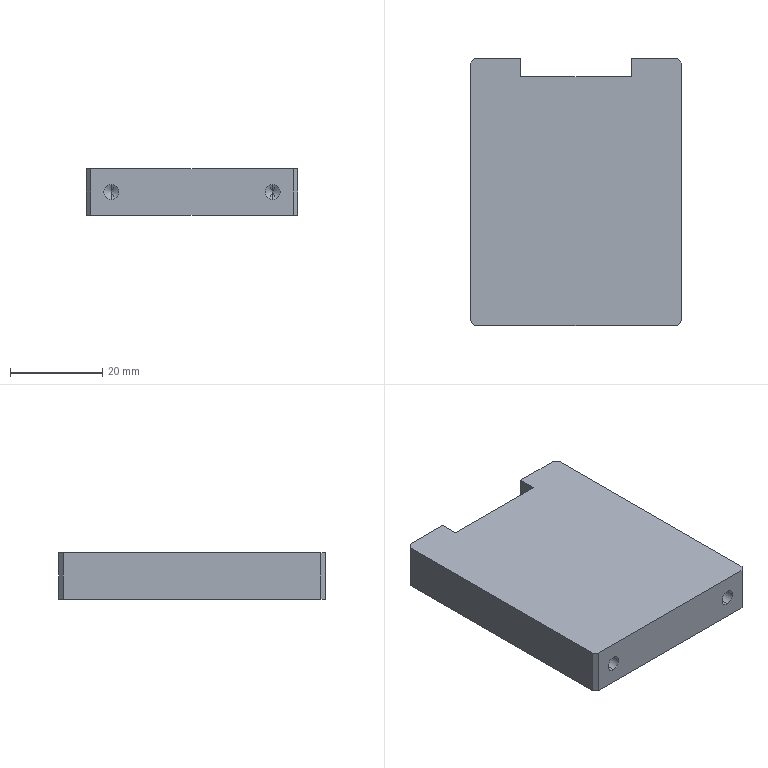Part | NX | features BREP 1 | 1 solid | 22 faces | box 46 x 58 x 10 mm | volume 25498 mm3 | plane 14 | cylinder 4 | cone 4 | commonest cylinder face diameters 3.3 x4
STEP:
#1=CARTESIAN_POINT('',(-17.5,-17.5,1.65));
#2=VERTEX_POINT('',#1);
#3=CARTESIAN_POINT('',(-17.5,-17.5,-1.65));
#4=VERTEX_POINT('',#3);
#5=CARTESIAN_POINT('',(-17.5,-17.5,0.));
#6=DIRECTION('',(0.,-1.,0.));
#7=DIRECTION('',(0.,0.,-1.));
#8=AXIS2_PLACEMENT_3D('',#5,#6,#7);
#9=CIRCLE('',#8,1.65);
#10=EDGE_CURVE('',#2,#4,#9,.T.);
#11=ORIENTED_EDGE('',*,*,#10,.F.);
#12=CARTESIAN_POINT('',(-17.5,-29.,1.65));
#13=VERTEX_POINT('',#12);
#14=CARTESIAN_POINT('',(-17.5,-29.,1.65));
#15=DIRECTION('',(0.,-1.,0.));
#16=VECTOR('',#15,1000.);
#17=LINE('',#14,#16);
#18=EDGE_CURVE('',#2,#13,#17,.T.);
#19=ORIENTED_EDGE('',*,*,#18,.T.);
#20=CARTESIAN_POINT('',(-17.5,-29.,-1.65));
#21=VERTEX_POINT('',#20);
#22=CARTESIAN_POINT('',(-17.5,-29.,0.));
#23=DIRECTION('',(0.,-1.,0.));
#24=DIRECTION('',(0.,0.,-1.));
#25=AXIS2_PLACEMENT_3D('',#22,#23,#24);
#26=CIRCLE('',#25,1.65);
#27=EDGE_CURVE('',#13,#21,#26,.T.);
#28=ORIENTED_EDGE('',*,*,#27,.T.);
#29=CARTESIAN_POINT('',(-17.5,-29.,-1.65));
#30=DIRECTION('',(0.,-1.,0.));
#31=VECTOR('',#30,1000.);
#32=LINE('',#29,#31);
#33=EDGE_CURVE('',#4,#21,#32,.T.);
#34=ORIENTED_EDGE('',*,*,#33,.F.);
#35=EDGE_LOOP('',(#11,#19,#28,#34));
#36=FACE_BOUND('',#35,.T.);
#37=CARTESIAN_POINT('',(-17.5,-29.,0.));
#38=DIRECTION('',(0.,-1.,0.));
#39=DIRECTION('',(0.,0.,-1.));
#40=AXIS2_PLACEMENT_3D('',#37,#38,#39);
#41=CYLINDRICAL_SURFACE('',#40,1.65);
#42=ADVANCED_FACE('',(#36),#41,.F.);
#43=CARTESIAN_POINT('',(-17.5,-16.509,0.));
#44=VERTEX_POINT('',#43);
#45=CARTESIAN_POINT('',(-17.5,-17.5,-1.65));
#46=DIRECTION('',(0.,-0.515,-0.8572));
#47=VECTOR('',#46,1000.);
#48=LINE('',#45,#47);
#49=EDGE_CURVE('',#44,#4,#48,.T.);
#50=ORIENTED_EDGE('',*,*,#49,.F.);
#51=CARTESIAN_POINT('',(-17.5,-17.5,1.65));
#52=DIRECTION('',(0.,-0.515,0.8572));
#53=VECTOR('',#52,1000.);
#54=LINE('',#51,#53);
#55=EDGE_CURVE('',#44,#2,#54,.T.);
#56=ORIENTED_EDGE('',*,*,#55,.T.);
#57=ORIENTED_EDGE('',*,*,#10,.T.);
#58=EDGE_LOOP('',(#50,#56,#57));
#59=FACE_BOUND('',#58,.T.);
#60=CARTESIAN_POINT('',(-17.5,-17.5,0.));
#61=DIRECTION('',(0.,-1.,0.));
#62=DIRECTION('',(0.,0.,-1.));
#63=AXIS2_PLACEMENT_3D('',#60,#61,#62);
#64=CONICAL_SURFACE('',#63,1.65,1.03);
#65=ADVANCED_FACE('',(#59),#64,.F.);
#66=CARTESIAN_POINT('',(17.5,-17.5,1.65));
#67=VERTEX_POINT('',#66);
#68=CARTESIAN_POINT('',(17.5,-17.5,-1.65));
#69=VERTEX_POINT('',#68);
#70=CARTESIAN_POINT('',(17.5,-17.5,0.));
#71=DIRECTION('',(0.,-1.,0.));
#72=DIRECTION('',(0.,0.,-1.));
#73=AXIS2_PLACEMENT_3D('',#70,#71,#72);
#74=CIRCLE('',#73,1.65);
#75=EDGE_CURVE('',#67,#69,#74,.T.);
#76=ORIENTED_EDGE('',*,*,#75,.F.);
#77=CARTESIAN_POINT('',(17.5,-29.,1.65));
#78=VERTEX_POINT('',#77);
#79=CARTESIAN_POINT('',(17.5,-29.,1.65));
#80=DIRECTION('',(0.,-1.,0.));
#81=VECTOR('',#80,1000.);
#82=LINE('',#79,#81);
#83=EDGE_CURVE('',#67,#78,#82,.T.);
#84=ORIENTED_EDGE('',*,*,#83,.T.);
#85=CARTESIAN_POINT('',(17.5,-29.,-1.65));
#86=VERTEX_POINT('',#85);
#87=CARTESIAN_POINT('',(17.5,-29.,0.));
#88=DIRECTION('',(0.,-1.,0.));
#89=DIRECTION('',(0.,0.,-1.));
#90=AXIS2_PLACEMENT_3D('',#87,#88,#89);
#91=CIRCLE('',#90,1.65);
#92=EDGE_CURVE('',#78,#86,#91,.T.);
#93=ORIENTED_EDGE('',*,*,#92,.T.);
#94=CARTESIAN_POINT('',(17.5,-29.,-1.65));
#95=DIRECTION('',(0.,-1.,0.));
#96=VECTOR('',#95,1000.);
#97=LINE('',#94,#96);
#98=EDGE_CURVE('',#69,#86,#97,.T.);
#99=ORIENTED_EDGE('',*,*,#98,.F.);
#100=EDGE_LOOP('',(#76,#84,#93,#99));
#101=FACE_BOUND('',#100,.T.);
#102=CARTESIAN_POINT('',(17.5,-29.,0.));
#103=DIRECTION('',(0.,-1.,0.));
#104=DIRECTION('',(0.,0.,-1.));
#105=AXIS2_PLACEMENT_3D('',#102,#103,#104);
#106=CYLINDRICAL_SURFACE('',#105,1.65);
#107=ADVANCED_FACE('',(#101),#106,.F.);
#108=CARTESIAN_POINT('',(17.5,-16.509,0.));
#109=VERTEX_POINT('',#108);
#110=CARTESIAN_POINT('',(17.5,-17.5,-1.65));
#111=DIRECTION('',(0.,-0.515,-0.8572));
#112=VECTOR('',#111,1000.);
#113=LINE('',#110,#112);
#114=EDGE_CURVE('',#109,#69,#113,.T.);
#115=ORIENTED_EDGE('',*,*,#114,.F.);
#116=CARTESIAN_POINT('',(17.5,-17.5,1.65));
#117=DIRECTION('',(0.,-0.515,0.8572));
#118=VECTOR('',#117,1000.);
#119=LINE('',#116,#118);
#120=EDGE_CURVE('',#109,#67,#119,.T.);
#121=ORIENTED_EDGE('',*,*,#120,.T.);
#122=ORIENTED_EDGE('',*,*,#75,.T.);
#123=EDGE_LOOP('',(#115,#121,#122));
#124=FACE_BOUND('',#123,.T.);
#125=CARTESIAN_POINT('',(17.5,-17.5,0.));
#126=DIRECTION('',(0.,-1.,0.));
#127=DIRECTION('',(0.,0.,-1.));
#128=AXIS2_PLACEMENT_3D('',#125,#126,#127);
#129=CONICAL_SURFACE('',#128,1.65,1.03);
#130=ADVANCED_FACE('',(#124),#129,.F.);
#131=CARTESIAN_POINT('',(22.,29.,5.));
#132=VERTEX_POINT('',#131);
#133=CARTESIAN_POINT('',(12.,29.,5.));
#134=VERTEX_POINT('',#133);
#135=CARTESIAN_POINT('',(23.,29.,5.));
#136=DIRECTION('',(-1.,0.,0.));
#137=VECTOR('',#136,1000.);
#138=LINE('',#135,#137);
#139=EDGE_CURVE('',#132,#134,#138,.T.);
#140=ORIENTED_EDGE('',*,*,#139,.F.);
#141=CARTESIAN_POINT('',(22.,29.,-5.));
#142=VERTEX_POINT('',#141);
#143=CARTESIAN_POINT('',(22.,29.,5.));
#144=DIRECTION('',(0.,0.,-1.));
#145=VECTOR('',#144,1000.);
#146=LINE('',#143,#145);
#147=EDGE_CURVE('',#132,#142,#146,.T.);
#148=ORIENTED_EDGE('',*,*,#147,.T.);
#149=CARTESIAN_POINT('',(12.,29.,-5.));
#150=VERTEX_POINT('',#149);
#151=CARTESIAN_POINT('',(23.,29.,-5.));
#152=DIRECTION('',(-1.,0.,0.));
#153=VECTOR('',#152,1000.);
#154=LINE('',#151,#153);
#155=EDGE_CURVE('',#142,#150,#154,.T.);
#156=ORIENTED_EDGE('',*,*,#155,.T.);
#157=CARTESIAN_POINT('',(12.,29.,-5.));
#158=DIRECTION('',(0.,0.,-1.));
#159=VECTOR('',#158,1000.);
#160=LINE('',#157,#159);
#161=EDGE_CURVE('',#134,#150,#160,.T.);
#162=ORIENTED_EDGE('',*,*,#161,.F.);
#163=EDGE_LOOP('',(#140,#148,#156,#162));
#164=FACE_BOUND('',#163,.T.);
#165=CARTESIAN_POINT('',(23.,29.,5.));
#166=DIRECTION('',(0.,-1.,0.));
#167=DIRECTION('',(0.,0.,-1.));
#168=AXIS2_PLACEMENT_3D('',#165,#166,#167);
#169=PLANE('',#168);
#170=ADVANCED_FACE('',(#164),#169,.F.);
#171=CARTESIAN_POINT('',(-23.,28.,-5.));
#172=VERTEX_POINT('',#171);
#173=CARTESIAN_POINT('',(-23.,-28.,-5.));
#174=VERTEX_POINT('',#173);
#175=CARTESIAN_POINT('',(-23.,-29.,-5.));
#176=DIRECTION('',(0.,-1.,0.));
#177=VECTOR('',#176,1000.);
#178=LINE('',#175,#177);
#179=EDGE_CURVE('',#172,#174,#178,.T.);
#180=ORIENTED_EDGE('',*,*,#179,.T.);
#181=CARTESIAN_POINT('',(-23.,-28.,5.));
#182=VERTEX_POINT('',#181);
#183=CARTESIAN_POINT('',(-23.,-28.,5.));
#184=DIRECTION('',(0.,0.,1.));
#185=VECTOR('',#184,1000.);
#186=LINE('',#183,#185);
#187=EDGE_CURVE('',#174,#182,#186,.T.);
#188=ORIENTED_EDGE('',*,*,#187,.T.);
#189=CARTESIAN_POINT('',(-23.,28.,5.));
#190=VERTEX_POINT('',#189);
#191=CARTESIAN_POINT('',(-23.,-29.,5.));
#192=DIRECTION('',(0.,-1.,0.));
#193=VECTOR('',#192,1000.);
#194=LINE('',#191,#193);
#195=EDGE_CURVE('',#190,#182,#194,.T.);
#196=ORIENTED_EDGE('',*,*,#195,.F.);
#197=CARTESIAN_POINT('',(-23.,28.,5.));
#198=DIRECTION('',(0.,0.,-1.));
#199=VECTOR('',#198,1000.);
#200=LINE('',#197,#199);
#201=EDGE_CURVE('',#190,#172,#200,.T.);
#202=ORIENTED_EDGE('',*,*,#201,.T.);
#203=EDGE_LOOP('',(#180,#188,#196,#202));
#204=FACE_BOUND('',#203,.T.);
#205=CARTESIAN_POINT('',(-23.,-29.,5.));
#206=DIRECTION('',(1.,0.,0.));
#207=DIRECTION('',(0.,1.,0.));
#208=AXIS2_PLACEMENT_3D('',#205,#206,#207);
#209=PLANE('',#208);
#210=ADVANCED_FACE('',(#204),#209,.F.);
#211=CARTESIAN_POINT('',(-22.,-29.,5.));
#212=VERTEX_POINT('',#211);
#213=CARTESIAN_POINT('',(22.,-29.,5.));
#214=VERTEX_POINT('',#213);
#215=CARTESIAN_POINT('',(23.,-29.,5.));
#216=DIRECTION('',(1.,0.,0.));
#217=VECTOR('',#216,1000.);
#218=LINE('',#215,#217);
#219=EDGE_CURVE('',#212,#214,#218,.T.);
#220=ORIENTED_EDGE('',*,*,#219,.F.);
#221=CARTESIAN_POINT('',(-22.,-29.,-5.));
#222=VERTEX_POINT('',#221);
#223=CARTESIAN_POINT('',(-22.,-29.,5.));
#224=DIRECTION('',(0.,0.,-1.));
#225=VECTOR('',#224,1000.);
#226=LINE('',#223,#225);
#227=EDGE_CURVE('',#212,#222,#226,.T.);
#228=ORIENTED_EDGE('',*,*,#227,.T.);
#229=CARTESIAN_POINT('',(22.,-29.,-5.));
#230=VERTEX_POINT('',#229);
#231=CARTESIAN_POINT('',(23.,-29.,-5.));
#232=DIRECTION('',(1.,0.,0.));
#233=VECTOR('',#232,1000.);
#234=LINE('',#231,#233);
#235=EDGE_CURVE('',#222,#230,#234,.T.);
#236=ORIENTED_EDGE('',*,*,#235,.T.);
#237=CARTESIAN_POINT('',(22.,-29.,5.));
#238=DIRECTION('',(0.,0.,1.));
#239=VECTOR('',#238,1000.);
#240=LINE('',#237,#239);
#241=EDGE_CURVE('',#230,#214,#240,.T.);
#242=ORIENTED_EDGE('',*,*,#241,.T.);
#243=EDGE_LOOP('',(#220,#228,#236,#242));
#244=FACE_BOUND('',#243,.T.);
#245=CARTESIAN_POINT('',(-17.5,-29.,0.));
#246=DIRECTION('',(0.,-1.,0.));
#247=DIRECTION('',(0.,0.,-1.));
#248=AXIS2_PLACEMENT_3D('',#245,#246,#247);
#249=CIRCLE('',#248,1.65);
#250=EDGE_CURVE('',#21,#13,#249,.T.);
#251=ORIENTED_EDGE('',*,*,#250,.F.);
#252=ORIENTED_EDGE('',*,*,#27,.F.);
#253=EDGE_LOOP('',(#251,#252));
#254=FACE_BOUND('',#253,.T.);
#255=CARTESIAN_POINT('',(17.5,-29.,0.));
#256=DIRECTION('',(0.,-1.,0.));
#257=DIRECTION('',(0.,0.,-1.));
#258=AXIS2_PLACEMENT_3D('',#255,#256,#257);
#259=CIRCLE('',#258,1.65);
#260=EDGE_CURVE('',#86,#78,#259,.T.);
#261=ORIENTED_EDGE('',*,*,#260,.F.);
#262=ORIENTED_EDGE('',*,*,#92,.F.);
#263=EDGE_LOOP('',(#261,#262));
#264=FACE_BOUND('',#263,.T.);
#265=CARTESIAN_POINT('',(23.,-29.,5.));
#266=DIRECTION('',(0.,1.,0.));
#267=DIRECTION('',(1.,0.,0.));
#268=AXIS2_PLACEMENT_3D('',#265,#266,#267);
#269=PLANE('',#268);
#270=ADVANCED_FACE('',(#244,#254,#264),#269,.F.);
#271=CARTESIAN_POINT('',(23.,-28.,5.));
#272=VERTEX_POINT('',#271);
#273=CARTESIAN_POINT('',(23.,28.,5.));
#274=VERTEX_POINT('',#273);
#275=CARTESIAN_POINT('',(23.,-29.,5.));
#276=DIRECTION('',(0.,1.,0.));
#277=VECTOR('',#276,1000.);
#278=LINE('',#275,#277);
#279=EDGE_CURVE('',#272,#274,#278,.T.);
#280=ORIENTED_EDGE('',*,*,#279,.F.);
#281=CARTESIAN_POINT('',(23.,-28.,-5.));
#282=VERTEX_POINT('',#281);
#283=CARTESIAN_POINT('',(23.,-28.,5.));
#284=DIRECTION('',(0.,0.,-1.));
#285=VECTOR('',#284,1000.);
#286=LINE('',#283,#285);
#287=EDGE_CURVE('',#272,#282,#286,.T.);
#288=ORIENTED_EDGE('',*,*,#287,.T.);
#289=CARTESIAN_POINT('',(23.,28.,-5.));
#290=VERTEX_POINT('',#289);
#291=CARTESIAN_POINT('',(23.,-29.,-5.));
#292=DIRECTION('',(0.,1.,0.));
#293=VECTOR('',#292,1000.);
#294=LINE('',#291,#293);
#295=EDGE_CURVE('',#282,#290,#294,.T.);
#296=ORIENTED_EDGE('',*,*,#295,.T.);
#297=CARTESIAN_POINT('',(23.,28.,5.));
#298=DIRECTION('',(0.,0.,1.));
#299=VECTOR('',#298,1000.);
#300=LINE('',#297,#299);
#301=EDGE_CURVE('',#290,#274,#300,.T.);
#302=ORIENTED_EDGE('',*,*,#301,.T.);
#303=EDGE_LOOP('',(#280,#288,#296,#302));
#304=FACE_BOUND('',#303,.T.);
#305=CARTESIAN_POINT('',(23.,-29.,5.));
#306=DIRECTION('',(-1.,0.,0.));
#307=DIRECTION('',(0.,0.,1.));
#308=AXIS2_PLACEMENT_3D('',#305,#306,#307);
#309=PLANE('',#308);
#310=ADVANCED_FACE('',(#304),#309,.F.);
#311=CARTESIAN_POINT('',(-12.,29.,-5.));
#312=VERTEX_POINT('',#311);
#313=CARTESIAN_POINT('',(-22.,29.,-5.));
#314=VERTEX_POINT('',#313);
#315=CARTESIAN_POINT('',(23.,29.,-5.));
#316=DIRECTION('',(-1.,0.,0.));
#317=VECTOR('',#316,1000.);
#318=LINE('',#315,#317);
#319=EDGE_CURVE('',#312,#314,#318,.T.);
#320=ORIENTED_EDGE('',*,*,#319,.T.);
#321=CARTESIAN_POINT('',(-22.,29.,5.));
#322=VERTEX_POINT('',#321);
#323=CARTESIAN_POINT('',(-22.,29.,5.));
#324=DIRECTION('',(0.,0.,1.));
#325=VECTOR('',#324,1000.);
#326=LINE('',#323,#325);
#327=EDGE_CURVE('',#314,#322,#326,.T.);
#328=ORIENTED_EDGE('',*,*,#327,.T.);
#329=CARTESIAN_POINT('',(-12.,29.,5.));
#330=VERTEX_POINT('',#329);
#331=CARTESIAN_POINT('',(23.,29.,5.));
#332=DIRECTION('',(-1.,0.,0.));
#333=VECTOR('',#332,1000.);
#334=LINE('',#331,#333);
#335=EDGE_CURVE('',#330,#322,#334,.T.);
#336=ORIENTED_EDGE('',*,*,#335,.F.);
#337=CARTESIAN_POINT('',(-12.,29.,-5.));
#338=DIRECTION('',(0.,0.,1.));
#339=VECTOR('',#338,1000.);
#340=LINE('',#337,#339);
#341=EDGE_CURVE('',#312,#330,#340,.T.);
#342=ORIENTED_EDGE('',*,*,#341,.F.);
#343=EDGE_LOOP('',(#320,#328,#336,#342));
#344=FACE_BOUND('',#343,.T.);
#345=CARTESIAN_POINT('',(23.,29.,5.));
#346=DIRECTION('',(0.,-1.,0.));
#347=DIRECTION('',(0.,0.,-1.));
#348=AXIS2_PLACEMENT_3D('',#345,#346,#347);
#349=PLANE('',#348);
#350=ADVANCED_FACE('',(#344),#349,.F.);
#351=ORIENTED_EDGE('',*,*,#195,.T.);
#352=CARTESIAN_POINT('',(-25.5,-25.5,5.));
#353=DIRECTION('',(0.7071,-0.7071,0.));
#354=VECTOR('',#353,1000.);
#355=LINE('',#352,#354);
#356=EDGE_CURVE('',#182,#212,#355,.T.);
#357=ORIENTED_EDGE('',*,*,#356,.T.);
#358=ORIENTED_EDGE('',*,*,#219,.T.);
#359=CARTESIAN_POINT('',(25.5,-25.5,5.));
#360=DIRECTION('',(0.7071,0.7071,0.));
#361=VECTOR('',#360,1000.);
#362=LINE('',#359,#361);
#363=EDGE_CURVE('',#214,#272,#362,.T.);
#364=ORIENTED_EDGE('',*,*,#363,.T.);
#365=ORIENTED_EDGE('',*,*,#279,.T.);
#366=CARTESIAN_POINT('',(25.5,25.5,5.));
#367=DIRECTION('',(-0.7071,0.7071,0.));
#368=VECTOR('',#367,1000.);
#369=LINE('',#366,#368);
#370=EDGE_CURVE('',#274,#132,#369,.T.);
#371=ORIENTED_EDGE('',*,*,#370,.T.);
#372=ORIENTED_EDGE('',*,*,#139,.T.);
#373=CARTESIAN_POINT('',(12.,25.,5.));
#374=VERTEX_POINT('',#373);
#375=CARTESIAN_POINT('',(12.,25.,5.));
#376=DIRECTION('',(0.,1.,0.));
#377=VECTOR('',#376,1000.);
#378=LINE('',#375,#377);
#379=EDGE_CURVE('',#374,#134,#378,.T.);
#380=ORIENTED_EDGE('',*,*,#379,.F.);
#381=CARTESIAN_POINT('',(-12.,25.,5.));
#382=VERTEX_POINT('',#381);
#383=CARTESIAN_POINT('',(-12.,25.,5.));
#384=DIRECTION('',(1.,0.,0.));
#385=VECTOR('',#384,1000.);
#386=LINE('',#383,#385);
#387=EDGE_CURVE('',#382,#374,#386,.T.);
#388=ORIENTED_EDGE('',*,*,#387,.F.);
#389=CARTESIAN_POINT('',(-12.,25.,5.));
#390=DIRECTION('',(0.,1.,0.));
#391=VECTOR('',#390,1000.);
#392=LINE('',#389,#391);
#393=EDGE_CURVE('',#382,#330,#392,.T.);
#394=ORIENTED_EDGE('',*,*,#393,.T.);
#395=ORIENTED_EDGE('',*,*,#335,.T.);
#396=CARTESIAN_POINT('',(-25.5,25.5,5.));
#397=DIRECTION('',(-0.7071,-0.7071,0.));
#398=VECTOR('',#397,1000.);
#399=LINE('',#396,#398);
#400=EDGE_CURVE('',#322,#190,#399,.T.);
#401=ORIENTED_EDGE('',*,*,#400,.T.);
#402=EDGE_LOOP('',(#351,#357,#358,#364,#365,#371,#372,#380,#388,#394,#395,#401));
#403=FACE_BOUND('',#402,.T.);
#404=CARTESIAN_POINT('',(0.,0.,5.));
#405=DIRECTION('',(0.,0.,1.));
#406=DIRECTION('',(1.,0.,0.));
#407=AXIS2_PLACEMENT_3D('',#404,#405,#406);
#408=PLANE('',#407);
#409=ADVANCED_FACE('',(#403),#408,.T.);
#410=ORIENTED_EDGE('',*,*,#235,.F.);
#411=CARTESIAN_POINT('',(-22.,-29.,-5.));
#412=DIRECTION('',(-0.7071,0.7071,0.));
#413=VECTOR('',#412,1000.);
#414=LINE('',#411,#413);
#415=EDGE_CURVE('',#222,#174,#414,.T.);
#416=ORIENTED_EDGE('',*,*,#415,.T.);
#417=ORIENTED_EDGE('',*,*,#179,.F.);
#418=CARTESIAN_POINT('',(-23.,28.,-5.));
#419=DIRECTION('',(0.7071,0.7071,0.));
#420=VECTOR('',#419,1000.);
#421=LINE('',#418,#420);
#422=EDGE_CURVE('',#172,#314,#421,.T.);
#423=ORIENTED_EDGE('',*,*,#422,.T.);
#424=ORIENTED_EDGE('',*,*,#319,.F.);
#425=CARTESIAN_POINT('',(-12.,25.,-5.));
#426=VERTEX_POINT('',#425);
#427=CARTESIAN_POINT('',(-12.,25.,-5.));
#428=DIRECTION('',(0.,1.,0.));
#429=VECTOR('',#428,1000.);
#430=LINE('',#427,#429);
#431=EDGE_CURVE('',#426,#312,#430,.T.);
#432=ORIENTED_EDGE('',*,*,#431,.F.);
#433=CARTESIAN_POINT('',(12.,25.,-5.));
#434=VERTEX_POINT('',#433);
#435=CARTESIAN_POINT('',(-12.,25.,-5.));
#436=DIRECTION('',(-1.,0.,0.));
#437=VECTOR('',#436,1000.);
#438=LINE('',#435,#437);
#439=EDGE_CURVE('',#434,#426,#438,.T.);
#440=ORIENTED_EDGE('',*,*,#439,.F.);
#441=CARTESIAN_POINT('',(12.,25.,-5.));
#442=DIRECTION('',(0.,1.,0.));
#443=VECTOR('',#442,1000.);
#444=LINE('',#441,#443);
#445=EDGE_CURVE('',#434,#150,#444,.T.);
#446=ORIENTED_EDGE('',*,*,#445,.T.);
#447=ORIENTED_EDGE('',*,*,#155,.F.);
#448=CARTESIAN_POINT('',(22.,29.,-5.));
#449=DIRECTION('',(0.7071,-0.7071,0.));
#450=VECTOR('',#449,1000.);
#451=LINE('',#448,#450);
#452=EDGE_CURVE('',#142,#290,#451,.T.);
#453=ORIENTED_EDGE('',*,*,#452,.T.);
#454=ORIENTED_EDGE('',*,*,#295,.F.);
#455=CARTESIAN_POINT('',(23.,-28.,-5.));
#456=DIRECTION('',(-0.7071,-0.7071,0.));
#457=VECTOR('',#456,1000.);
#458=LINE('',#455,#457);
#459=EDGE_CURVE('',#282,#230,#458,.T.);
#460=ORIENTED_EDGE('',*,*,#459,.T.);
#461=EDGE_LOOP('',(#410,#416,#417,#423,#424,#432,#440,#446,#447,#453,#454,#460));
#462=FACE_BOUND('',#461,.T.);
#463=CARTESIAN_POINT('',(0.,0.,-5.));
#464=DIRECTION('',(0.,0.,1.));
#465=DIRECTION('',(1.,0.,0.));
#466=AXIS2_PLACEMENT_3D('',#463,#464,#465);
#467=PLANE('',#466);
#468=ADVANCED_FACE('',(#462),#467,.F.);
#469=ORIENTED_EDGE('',*,*,#161,.T.);
#470=ORIENTED_EDGE('',*,*,#445,.F.);
#471=CARTESIAN_POINT('',(12.,25.,-5.));
#472=DIRECTION('',(0.,0.,-1.));
#473=VECTOR('',#472,1000.);
#474=LINE('',#471,#473);
#475=EDGE_CURVE('',#374,#434,#474,.T.);
#476=ORIENTED_EDGE('',*,*,#475,.F.);
#477=ORIENTED_EDGE('',*,*,#379,.T.);
#478=EDGE_LOOP('',(#469,#470,#476,#477));
#479=FACE_BOUND('',#478,.T.);
#480=CARTESIAN_POINT('',(12.,25.,-5.));
#481=DIRECTION('',(1.,0.,0.));
#482=DIRECTION('',(0.,1.,0.));
#483=AXIS2_PLACEMENT_3D('',#480,#481,#482);
#484=PLANE('',#483);
#485=ADVANCED_FACE('',(#479),#484,.F.);
#486=ORIENTED_EDGE('',*,*,#341,.T.);
#487=ORIENTED_EDGE('',*,*,#393,.F.);
#488=CARTESIAN_POINT('',(-12.,25.,-5.));
#489=DIRECTION('',(0.,0.,1.));
#490=VECTOR('',#489,1000.);
#491=LINE('',#488,#490);
#492=EDGE_CURVE('',#426,#382,#491,.T.);
#493=ORIENTED_EDGE('',*,*,#492,.F.);
#494=ORIENTED_EDGE('',*,*,#431,.T.);
#495=EDGE_LOOP('',(#486,#487,#493,#494));
#496=FACE_BOUND('',#495,.T.);
#497=CARTESIAN_POINT('',(-12.,25.,-5.));
#498=DIRECTION('',(-1.,0.,0.));
#499=DIRECTION('',(0.,0.,1.));
#500=AXIS2_PLACEMENT_3D('',#497,#498,#499);
#501=PLANE('',#500);
#502=ADVANCED_FACE('',(#496),#501,.F.);
#503=ORIENTED_EDGE('',*,*,#475,.T.);
#504=ORIENTED_EDGE('',*,*,#439,.T.);
#505=ORIENTED_EDGE('',*,*,#492,.T.);
#506=ORIENTED_EDGE('',*,*,#387,.T.);
#507=EDGE_LOOP('',(#503,#504,#505,#506));
#508=FACE_BOUND('',#507,.T.);
#509=CARTESIAN_POINT('',(0.,25.,0.));
#510=DIRECTION('',(0.,1.,0.));
#511=DIRECTION('',(1.,0.,0.));
#512=AXIS2_PLACEMENT_3D('',#509,#510,#511);
#513=PLANE('',#512);
#514=ADVANCED_FACE('',(#508),#513,.T.);
#515=ORIENTED_EDGE('',*,*,#356,.F.);
#516=ORIENTED_EDGE('',*,*,#187,.F.);
#517=ORIENTED_EDGE('',*,*,#415,.F.);
#518=ORIENTED_EDGE('',*,*,#227,.F.);
#519=EDGE_LOOP('',(#515,#516,#517,#518));
#520=FACE_BOUND('',#519,.T.);
#521=CARTESIAN_POINT('',(-22.,-29.,5.));
#522=DIRECTION('',(0.7071,0.7071,0.));
#523=DIRECTION('',(0.,0.,-1.));
#524=AXIS2_PLACEMENT_3D('',#521,#522,#523);
#525=PLANE('',#524);
#526=ADVANCED_FACE('',(#520),#525,.F.);
#527=ORIENTED_EDGE('',*,*,#400,.F.);
#528=ORIENTED_EDGE('',*,*,#327,.F.);
#529=ORIENTED_EDGE('',*,*,#422,.F.);
#530=ORIENTED_EDGE('',*,*,#201,.F.);
#531=EDGE_LOOP('',(#527,#528,#529,#530));
#532=FACE_BOUND('',#531,.T.);
#533=CARTESIAN_POINT('',(-23.,28.,5.));
#534=DIRECTION('',(0.7071,-0.7071,0.));
#535=DIRECTION('',(0.,0.,-1.));
#536=AXIS2_PLACEMENT_3D('',#533,#534,#535);
#537=PLANE('',#536);
#538=ADVANCED_FACE('',(#532),#537,.F.);
#539=ORIENTED_EDGE('',*,*,#363,.F.);
#540=ORIENTED_EDGE('',*,*,#241,.F.);
#541=ORIENTED_EDGE('',*,*,#459,.F.);
#542=ORIENTED_EDGE('',*,*,#287,.F.);
#543=EDGE_LOOP('',(#539,#540,#541,#542));
#544=FACE_BOUND('',#543,.T.);
#545=CARTESIAN_POINT('',(23.,-28.,5.));
#546=DIRECTION('',(-0.7071,0.7071,0.));
#547=DIRECTION('',(0.,0.,1.));
#548=AXIS2_PLACEMENT_3D('',#545,#546,#547);
#549=PLANE('',#548);
#550=ADVANCED_FACE('',(#544),#549,.F.);
#551=ORIENTED_EDGE('',*,*,#370,.F.);
#552=ORIENTED_EDGE('',*,*,#301,.F.);
#553=ORIENTED_EDGE('',*,*,#452,.F.);
#554=ORIENTED_EDGE('',*,*,#147,.F.);
#555=EDGE_LOOP('',(#551,#552,#553,#554));
#556=FACE_BOUND('',#555,.T.);
#557=CARTESIAN_POINT('',(22.,29.,5.));
#558=DIRECTION('',(-0.7071,-0.7071,0.));
#559=DIRECTION('',(-0.7071,0.7071,0.));
#560=AXIS2_PLACEMENT_3D('',#557,#558,#559);
#561=PLANE('',#560);
#562=ADVANCED_FACE('',(#556),#561,.F.);
#563=ORIENTED_EDGE('',*,*,#120,.F.);
#564=ORIENTED_EDGE('',*,*,#114,.T.);
#565=CARTESIAN_POINT('',(17.5,-17.5,0.));
#566=DIRECTION('',(0.,-1.,0.));
#567=DIRECTION('',(0.,0.,-1.));
#568=AXIS2_PLACEMENT_3D('',#565,#566,#567);
#569=CIRCLE('',#568,1.65);
#570=EDGE_CURVE('',#69,#67,#569,.T.);
#571=ORIENTED_EDGE('',*,*,#570,.T.);
#572=EDGE_LOOP('',(#563,#564,#571));
#573=FACE_BOUND('',#572,.T.);
#574=CARTESIAN_POINT('',(17.5,-17.5,0.));
#575=DIRECTION('',(0.,-1.,0.));
#576=DIRECTION('',(0.,0.,-1.));
#577=AXIS2_PLACEMENT_3D('',#574,#575,#576);
#578=CONICAL_SURFACE('',#577,1.65,1.03);
#579=ADVANCED_FACE('',(#573),#578,.F.);
#580=ORIENTED_EDGE('',*,*,#83,.F.);
#581=ORIENTED_EDGE('',*,*,#570,.F.);
#582=ORIENTED_EDGE('',*,*,#98,.T.);
#583=ORIENTED_EDGE('',*,*,#260,.T.);
#584=EDGE_LOOP('',(#580,#581,#582,#583));
#585=FACE_BOUND('',#584,.T.);
#586=CARTESIAN_POINT('',(17.5,-29.,0.));
#587=DIRECTION('',(0.,-1.,0.));
#588=DIRECTION('',(0.,0.,-1.));
#589=AXIS2_PLACEMENT_3D('',#586,#587,#588);
#590=CYLINDRICAL_SURFACE('',#589,1.65);
#591=ADVANCED_FACE('',(#585),#590,.F.);
#592=ORIENTED_EDGE('',*,*,#55,.F.);
#593=ORIENTED_EDGE('',*,*,#49,.T.);
#594=CARTESIAN_POINT('',(-17.5,-17.5,0.));
#595=DIRECTION('',(0.,-1.,0.));
#596=DIRECTION('',(0.,0.,-1.));
#597=AXIS2_PLACEMENT_3D('',#594,#595,#596);
#598=CIRCLE('',#597,1.65);
#599=EDGE_CURVE('',#4,#2,#598,.T.);
#600=ORIENTED_EDGE('',*,*,#599,.T.);
#601=EDGE_LOOP('',(#592,#593,#600));
#602=FACE_BOUND('',#601,.T.);
#603=CARTESIAN_POINT('',(-17.5,-17.5,0.));
#604=DIRECTION('',(0.,-1.,0.));
#605=DIRECTION('',(0.,0.,-1.));
#606=AXIS2_PLACEMENT_3D('',#603,#604,#605);
#607=CONICAL_SURFACE('',#606,1.65,1.03);
#608=ADVANCED_FACE('',(#602),#607,.F.);
#609=ORIENTED_EDGE('',*,*,#18,.F.);
#610=ORIENTED_EDGE('',*,*,#599,.F.);
#611=ORIENTED_EDGE('',*,*,#33,.T.);
#612=ORIENTED_EDGE('',*,*,#250,.T.);
#613=EDGE_LOOP('',(#609,#610,#611,#612));
#614=FACE_BOUND('',#613,.T.);
#615=CARTESIAN_POINT('',(-17.5,-29.,0.));
#616=DIRECTION('',(0.,-1.,0.));
#617=DIRECTION('',(0.,0.,-1.));
#618=AXIS2_PLACEMENT_3D('',#615,#616,#617);
#619=CYLINDRICAL_SURFACE('',#618,1.65);
#620=ADVANCED_FACE('',(#614),#619,.F.);
#621=CLOSED_SHELL('',(#42,#65,#107,#130,#170,#210,#270,#310,#350,#409,#468,#485,#502,#514,#526,#538,#550,#562,#579,#591,#608,#620));
#622=MANIFOLD_SOLID_BREP('',#621);
#623=(LENGTH_UNIT()NAMED_UNIT(*)SI_UNIT(.MILLI.,.METRE.));
#624=UNCERTAINTY_MEASURE_WITH_UNIT(LENGTH_MEASURE(0.00001),#623,'','');
#625=(NAMED_UNIT(*)PLANE_ANGLE_UNIT()SI_UNIT($,.RADIAN.));
#626=(NAMED_UNIT(*)SI_UNIT($,.STERADIAN.)SOLID_ANGLE_UNIT());
#627=(GEOMETRIC_REPRESENTATION_CONTEXT(3)GLOBAL_UNCERTAINTY_ASSIGNED_CONTEXT((#624))GLOBAL_UNIT_ASSIGNED_CONTEXT((#623,#625,#626))REPRESENTATION_CONTEXT('',''));
#628=ADVANCED_BREP_SHAPE_REPRESENTATION('',(#622),#627);